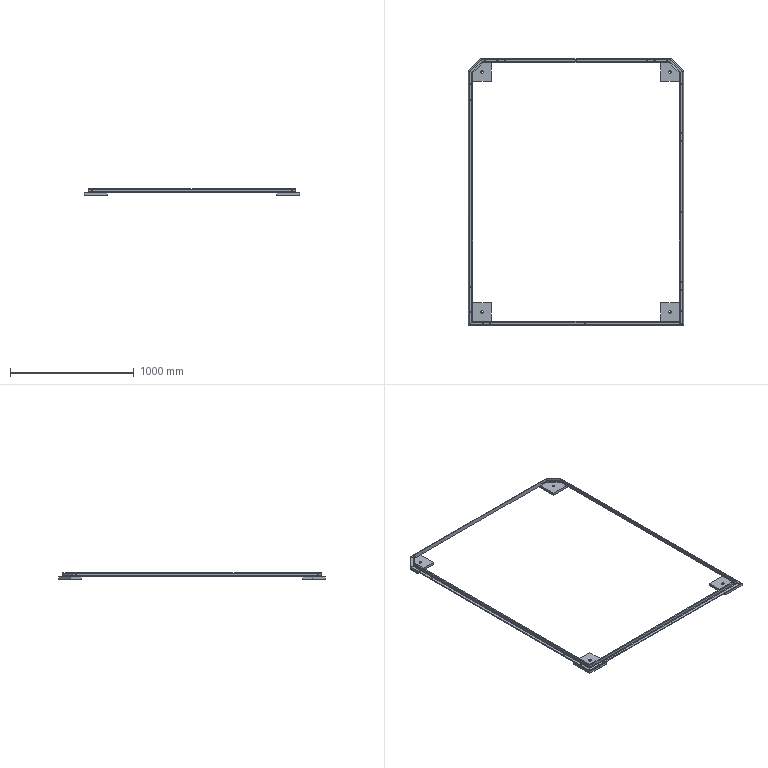Part | SolidWorks | features ICE 7, WeldMemberFeat 1, WeldmentFeature 1 | 10 solids | 158 faces | box 1740 x 2160 x 55 mm | volume 4890635 mm3 | cylinder 96 | plane 62 | commonest cylinder face diameters 9 x70 10 x18 20 x8